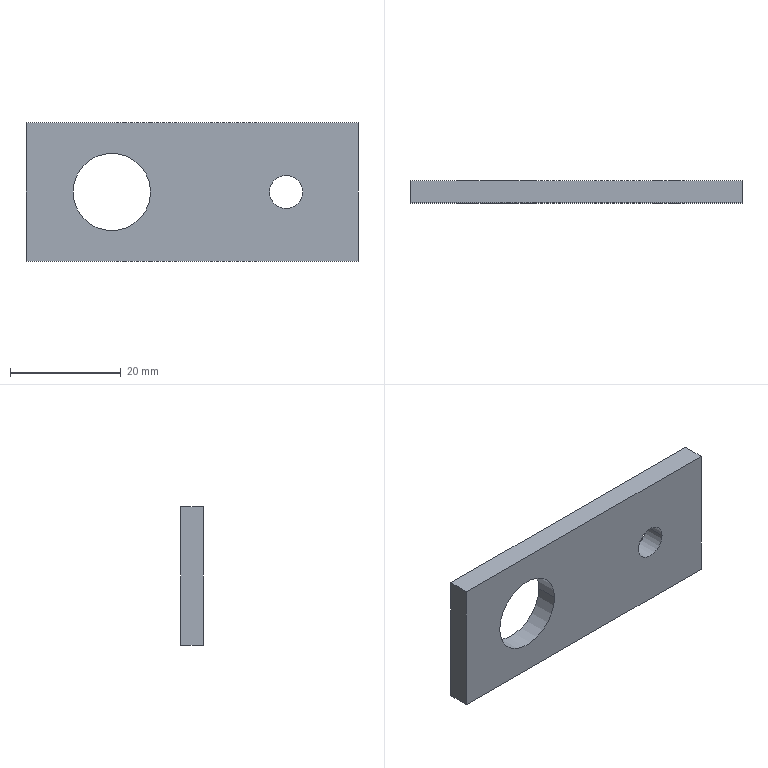Part | STEP file | Connecting plate | 1 solid | 10 faces | box 60 x 4 x 25 mm | volume 5271 mm3 | plane 6 | cylinder 4 | commonest cylinder face diameters 6 x2 14 x2
STEP:
#1=CARTESIAN_POINT('',(-37.49,0.,12.5));
#2=VERTEX_POINT('',#1);
#3=CARTESIAN_POINT('',(-51.49,0.,12.5));
#4=VERTEX_POINT('',#3);
#5=CARTESIAN_POINT('',(-44.49,0.,12.5));
#6=DIRECTION('',(0.,1.,0.));
#7=DIRECTION('',(1.,0.,0.));
#8=AXIS2_PLACEMENT_3D('',#5,#6,#7);
#9=CIRCLE('',#8,7.);
#10=EDGE_CURVE('',#2,#4,#9,.T.);
#11=ORIENTED_EDGE('',*,*,#10,.F.);
#12=CARTESIAN_POINT('',(-37.49,4.,12.5));
#13=VERTEX_POINT('',#12);
#14=CARTESIAN_POINT('',(-37.49,-0.001,12.5));
#15=DIRECTION('',(0.,1.,0.));
#16=VECTOR('',#15,1000.);
#17=LINE('',#14,#16);
#18=EDGE_CURVE('',#2,#13,#17,.T.);
#19=ORIENTED_EDGE('',*,*,#18,.T.);
#20=CARTESIAN_POINT('',(-51.49,4.,12.5));
#21=VERTEX_POINT('',#20);
#22=CARTESIAN_POINT('',(-44.49,4.,12.5));
#23=DIRECTION('',(0.,1.,0.));
#24=DIRECTION('',(-1.,0.,0.));
#25=AXIS2_PLACEMENT_3D('',#22,#23,#24);
#26=CIRCLE('',#25,7.);
#27=EDGE_CURVE('',#13,#21,#26,.T.);
#28=ORIENTED_EDGE('',*,*,#27,.T.);
#29=CARTESIAN_POINT('',(-51.49,-0.001,12.5));
#30=DIRECTION('',(0.,1.,0.));
#31=VECTOR('',#30,1000.);
#32=LINE('',#29,#31);
#33=EDGE_CURVE('',#4,#21,#32,.T.);
#34=ORIENTED_EDGE('',*,*,#33,.F.);
#35=EDGE_LOOP('',(#11,#19,#28,#34));
#36=FACE_OUTER_BOUND('',#35,.T.);
#37=CARTESIAN_POINT('',(-44.49,-0.001,12.5));
#38=DIRECTION('',(0.,1.,0.));
#39=DIRECTION('',(-1.,0.,0.));
#40=AXIS2_PLACEMENT_3D('',#37,#38,#39);
#41=CYLINDRICAL_SURFACE('',#40,7.);
#42=ADVANCED_FACE('',(#36),#41,.F.);
#43=CARTESIAN_POINT('',(-10.,0.,12.5));
#44=VERTEX_POINT('',#43);
#45=CARTESIAN_POINT('',(-16.,0.,12.5));
#46=VERTEX_POINT('',#45);
#47=CARTESIAN_POINT('',(-13.,0.,12.5));
#48=DIRECTION('',(0.,1.,0.));
#49=DIRECTION('',(1.,0.,0.));
#50=AXIS2_PLACEMENT_3D('',#47,#48,#49);
#51=CIRCLE('',#50,3.);
#52=EDGE_CURVE('',#44,#46,#51,.T.);
#53=ORIENTED_EDGE('',*,*,#52,.F.);
#54=CARTESIAN_POINT('',(-10.,4.,12.5));
#55=VERTEX_POINT('',#54);
#56=CARTESIAN_POINT('',(-10.,-0.001,12.5));
#57=DIRECTION('',(0.,1.,0.));
#58=VECTOR('',#57,1000.);
#59=LINE('',#56,#58);
#60=EDGE_CURVE('',#44,#55,#59,.T.);
#61=ORIENTED_EDGE('',*,*,#60,.T.);
#62=CARTESIAN_POINT('',(-16.,4.,12.5));
#63=VERTEX_POINT('',#62);
#64=CARTESIAN_POINT('',(-13.,4.,12.5));
#65=DIRECTION('',(0.,1.,0.));
#66=DIRECTION('',(-1.,0.,0.));
#67=AXIS2_PLACEMENT_3D('',#64,#65,#66);
#68=CIRCLE('',#67,3.);
#69=EDGE_CURVE('',#55,#63,#68,.T.);
#70=ORIENTED_EDGE('',*,*,#69,.T.);
#71=CARTESIAN_POINT('',(-16.,-0.001,12.5));
#72=DIRECTION('',(0.,1.,0.));
#73=VECTOR('',#72,1000.);
#74=LINE('',#71,#73);
#75=EDGE_CURVE('',#46,#63,#74,.T.);
#76=ORIENTED_EDGE('',*,*,#75,.F.);
#77=EDGE_LOOP('',(#53,#61,#70,#76));
#78=FACE_OUTER_BOUND('',#77,.T.);
#79=CARTESIAN_POINT('',(-13.,-0.001,12.5));
#80=DIRECTION('',(0.,1.,0.));
#81=DIRECTION('',(-1.,0.,0.));
#82=AXIS2_PLACEMENT_3D('',#79,#80,#81);
#83=CYLINDRICAL_SURFACE('',#82,3.);
#84=ADVANCED_FACE('',(#78),#83,.F.);
#85=CARTESIAN_POINT('',(-44.49,4.,12.5));
#86=DIRECTION('',(0.,1.,0.));
#87=DIRECTION('',(-1.,0.,0.));
#88=AXIS2_PLACEMENT_3D('',#85,#86,#87);
#89=CIRCLE('',#88,7.);
#90=EDGE_CURVE('',#21,#13,#89,.T.);
#91=ORIENTED_EDGE('',*,*,#90,.F.);
#92=ORIENTED_EDGE('',*,*,#27,.F.);
#93=EDGE_LOOP('',(#91,#92));
#94=FACE_BOUND('',#93,.T.);
#95=CARTESIAN_POINT('',(-13.,4.,12.5));
#96=DIRECTION('',(0.,1.,0.));
#97=DIRECTION('',(-1.,0.,0.));
#98=AXIS2_PLACEMENT_3D('',#95,#96,#97);
#99=CIRCLE('',#98,3.);
#100=EDGE_CURVE('',#63,#55,#99,.T.);
#101=ORIENTED_EDGE('',*,*,#100,.F.);
#102=ORIENTED_EDGE('',*,*,#69,.F.);
#103=EDGE_LOOP('',(#101,#102));
#104=FACE_BOUND('',#103,.T.);
#105=CARTESIAN_POINT('',(0.,4.,0.));
#106=VERTEX_POINT('',#105);
#107=CARTESIAN_POINT('',(-60.,4.,0.));
#108=VERTEX_POINT('',#107);
#109=CARTESIAN_POINT('',(0.,4.,0.));
#110=DIRECTION('',(-1.,0.,0.));
#111=VECTOR('',#110,1000.);
#112=LINE('',#109,#111);
#113=EDGE_CURVE('',#106,#108,#112,.T.);
#114=ORIENTED_EDGE('',*,*,#113,.T.);
#115=CARTESIAN_POINT('',(-60.,4.,25.));
#116=VERTEX_POINT('',#115);
#117=CARTESIAN_POINT('',(-60.,4.,25.));
#118=DIRECTION('',(0.,0.,-1.));
#119=VECTOR('',#118,1000.);
#120=LINE('',#117,#119);
#121=EDGE_CURVE('',#116,#108,#120,.T.);
#122=ORIENTED_EDGE('',*,*,#121,.F.);
#123=CARTESIAN_POINT('',(0.,4.,25.));
#124=VERTEX_POINT('',#123);
#125=CARTESIAN_POINT('',(0.,4.,25.));
#126=DIRECTION('',(-1.,0.,0.));
#127=VECTOR('',#126,1000.);
#128=LINE('',#125,#127);
#129=EDGE_CURVE('',#124,#116,#128,.T.);
#130=ORIENTED_EDGE('',*,*,#129,.F.);
#131=CARTESIAN_POINT('',(0.,4.,25.));
#132=DIRECTION('',(0.,0.,-1.));
#133=VECTOR('',#132,1000.);
#134=LINE('',#131,#133);
#135=EDGE_CURVE('',#124,#106,#134,.T.);
#136=ORIENTED_EDGE('',*,*,#135,.T.);
#137=EDGE_LOOP('',(#114,#122,#130,#136));
#138=FACE_OUTER_BOUND('',#137,.T.);
#139=CARTESIAN_POINT('',(0.,4.,25.));
#140=DIRECTION('',(0.,-1.,0.));
#141=DIRECTION('',(1.,0.,0.));
#142=AXIS2_PLACEMENT_3D('',#139,#140,#141);
#143=PLANE('',#142);
#144=ADVANCED_FACE('',(#94,#104,#138),#143,.F.);
#145=CARTESIAN_POINT('',(-60.,0.,0.));
#146=VERTEX_POINT('',#145);
#147=CARTESIAN_POINT('',(-60.,0.,0.));
#148=DIRECTION('',(0.,1.,0.));
#149=VECTOR('',#148,1000.);
#150=LINE('',#147,#149);
#151=EDGE_CURVE('',#146,#108,#150,.T.);
#152=ORIENTED_EDGE('',*,*,#151,.F.);
#153=CARTESIAN_POINT('',(-60.,0.,25.));
#154=VERTEX_POINT('',#153);
#155=CARTESIAN_POINT('',(-60.,0.,25.));
#156=DIRECTION('',(0.,0.,-1.));
#157=VECTOR('',#156,1000.);
#158=LINE('',#155,#157);
#159=EDGE_CURVE('',#154,#146,#158,.T.);
#160=ORIENTED_EDGE('',*,*,#159,.F.);
#161=CARTESIAN_POINT('',(-60.,0.,25.));
#162=DIRECTION('',(0.,1.,0.));
#163=VECTOR('',#162,1000.);
#164=LINE('',#161,#163);
#165=EDGE_CURVE('',#154,#116,#164,.T.);
#166=ORIENTED_EDGE('',*,*,#165,.T.);
#167=ORIENTED_EDGE('',*,*,#121,.T.);
#168=EDGE_LOOP('',(#152,#160,#166,#167));
#169=FACE_OUTER_BOUND('',#168,.T.);
#170=CARTESIAN_POINT('',(-60.,0.,25.));
#171=DIRECTION('',(-1.,0.,0.));
#172=DIRECTION('',(0.,0.,1.));
#173=AXIS2_PLACEMENT_3D('',#170,#171,#172);
#174=PLANE('',#173);
#175=ADVANCED_FACE('',(#169),#174,.T.);
#176=CARTESIAN_POINT('',(-44.49,0.,12.5));
#177=DIRECTION('',(0.,1.,0.));
#178=DIRECTION('',(1.,0.,0.));
#179=AXIS2_PLACEMENT_3D('',#176,#177,#178);
#180=CIRCLE('',#179,7.);
#181=EDGE_CURVE('',#4,#2,#180,.T.);
#182=ORIENTED_EDGE('',*,*,#181,.T.);
#183=ORIENTED_EDGE('',*,*,#10,.T.);
#184=EDGE_LOOP('',(#182,#183));
#185=FACE_BOUND('',#184,.T.);
#186=CARTESIAN_POINT('',(-13.,0.,12.5));
#187=DIRECTION('',(0.,1.,0.));
#188=DIRECTION('',(1.,0.,0.));
#189=AXIS2_PLACEMENT_3D('',#186,#187,#188);
#190=CIRCLE('',#189,3.);
#191=EDGE_CURVE('',#46,#44,#190,.T.);
#192=ORIENTED_EDGE('',*,*,#191,.T.);
#193=ORIENTED_EDGE('',*,*,#52,.T.);
#194=EDGE_LOOP('',(#192,#193));
#195=FACE_BOUND('',#194,.T.);
#196=CARTESIAN_POINT('',(0.,0.,0.));
#197=VERTEX_POINT('',#196);
#198=CARTESIAN_POINT('',(0.,0.,0.));
#199=DIRECTION('',(-1.,0.,0.));
#200=VECTOR('',#199,1000.);
#201=LINE('',#198,#200);
#202=EDGE_CURVE('',#197,#146,#201,.T.);
#203=ORIENTED_EDGE('',*,*,#202,.F.);
#204=CARTESIAN_POINT('',(0.,0.,25.));
#205=VERTEX_POINT('',#204);
#206=CARTESIAN_POINT('',(0.,0.,25.));
#207=DIRECTION('',(0.,0.,-1.));
#208=VECTOR('',#207,1000.);
#209=LINE('',#206,#208);
#210=EDGE_CURVE('',#205,#197,#209,.T.);
#211=ORIENTED_EDGE('',*,*,#210,.F.);
#212=CARTESIAN_POINT('',(0.,0.,25.));
#213=DIRECTION('',(-1.,0.,0.));
#214=VECTOR('',#213,1000.);
#215=LINE('',#212,#214);
#216=EDGE_CURVE('',#205,#154,#215,.T.);
#217=ORIENTED_EDGE('',*,*,#216,.T.);
#218=ORIENTED_EDGE('',*,*,#159,.T.);
#219=EDGE_LOOP('',(#203,#211,#217,#218));
#220=FACE_OUTER_BOUND('',#219,.T.);
#221=CARTESIAN_POINT('',(0.,0.,25.));
#222=DIRECTION('',(0.,-1.,0.));
#223=DIRECTION('',(1.,0.,0.));
#224=AXIS2_PLACEMENT_3D('',#221,#222,#223);
#225=PLANE('',#224);
#226=ADVANCED_FACE('',(#185,#195,#220),#225,.T.);
#227=CARTESIAN_POINT('',(0.,4.,0.));
#228=DIRECTION('',(0.,-1.,0.));
#229=VECTOR('',#228,1000.);
#230=LINE('',#227,#229);
#231=EDGE_CURVE('',#106,#197,#230,.T.);
#232=ORIENTED_EDGE('',*,*,#231,.F.);
#233=ORIENTED_EDGE('',*,*,#135,.F.);
#234=CARTESIAN_POINT('',(0.,4.,25.));
#235=DIRECTION('',(0.,-1.,0.));
#236=VECTOR('',#235,1000.);
#237=LINE('',#234,#236);
#238=EDGE_CURVE('',#124,#205,#237,.T.);
#239=ORIENTED_EDGE('',*,*,#238,.T.);
#240=ORIENTED_EDGE('',*,*,#210,.T.);
#241=EDGE_LOOP('',(#232,#233,#239,#240));
#242=FACE_OUTER_BOUND('',#241,.T.);
#243=CARTESIAN_POINT('',(0.,4.,25.));
#244=DIRECTION('',(1.,0.,0.));
#245=DIRECTION('',(0.,1.,0.));
#246=AXIS2_PLACEMENT_3D('',#243,#244,#245);
#247=PLANE('',#246);
#248=ADVANCED_FACE('',(#242),#247,.T.);
#249=ORIENTED_EDGE('',*,*,#129,.T.);
#250=ORIENTED_EDGE('',*,*,#165,.F.);
#251=ORIENTED_EDGE('',*,*,#216,.F.);
#252=ORIENTED_EDGE('',*,*,#238,.F.);
#253=EDGE_LOOP('',(#249,#250,#251,#252));
#254=FACE_OUTER_BOUND('',#253,.T.);
#255=CARTESIAN_POINT('',(0.,0.,25.));
#256=DIRECTION('',(0.,0.,-1.));
#257=DIRECTION('',(-1.,0.,0.));
#258=AXIS2_PLACEMENT_3D('',#255,#256,#257);
#259=PLANE('',#258);
#260=ADVANCED_FACE('',(#254),#259,.F.);
#261=ORIENTED_EDGE('',*,*,#113,.F.);
#262=ORIENTED_EDGE('',*,*,#231,.T.);
#263=ORIENTED_EDGE('',*,*,#202,.T.);
#264=ORIENTED_EDGE('',*,*,#151,.T.);
#265=EDGE_LOOP('',(#261,#262,#263,#264));
#266=FACE_OUTER_BOUND('',#265,.T.);
#267=CARTESIAN_POINT('',(0.,0.,0.));
#268=DIRECTION('',(0.,0.,-1.));
#269=DIRECTION('',(-1.,0.,0.));
#270=AXIS2_PLACEMENT_3D('',#267,#268,#269);
#271=PLANE('',#270);
#272=ADVANCED_FACE('',(#266),#271,.T.);
#273=ORIENTED_EDGE('',*,*,#60,.F.);
#274=ORIENTED_EDGE('',*,*,#191,.F.);
#275=ORIENTED_EDGE('',*,*,#75,.T.);
#276=ORIENTED_EDGE('',*,*,#100,.T.);
#277=EDGE_LOOP('',(#273,#274,#275,#276));
#278=FACE_OUTER_BOUND('',#277,.T.);
#279=CARTESIAN_POINT('',(-13.,-0.001,12.5));
#280=DIRECTION('',(0.,1.,0.));
#281=DIRECTION('',(-1.,0.,0.));
#282=AXIS2_PLACEMENT_3D('',#279,#280,#281);
#283=CYLINDRICAL_SURFACE('',#282,3.);
#284=ADVANCED_FACE('',(#278),#283,.F.);
#285=ORIENTED_EDGE('',*,*,#18,.F.);
#286=ORIENTED_EDGE('',*,*,#181,.F.);
#287=ORIENTED_EDGE('',*,*,#33,.T.);
#288=ORIENTED_EDGE('',*,*,#90,.T.);
#289=EDGE_LOOP('',(#285,#286,#287,#288));
#290=FACE_OUTER_BOUND('',#289,.T.);
#291=CARTESIAN_POINT('',(-44.49,-0.001,12.5));
#292=DIRECTION('',(0.,1.,0.));
#293=DIRECTION('',(-1.,0.,0.));
#294=AXIS2_PLACEMENT_3D('',#291,#292,#293);
#295=CYLINDRICAL_SURFACE('',#294,7.);
#296=ADVANCED_FACE('',(#290),#295,.F.);
#297=CLOSED_SHELL('',(#42,#84,#144,#175,#226,#248,#260,#272,#284,#296));
#298=MANIFOLD_SOLID_BREP('',#297);
#299=CARTESIAN_POINT('',(0.,0.,0.));
#300=DIRECTION('',(0.,0.,1.));
#301=DIRECTION('',(1.,0.,0.));
#302=AXIS2_PLACEMENT_3D('',#299,#300,#301);
#303=(LENGTH_UNIT()NAMED_UNIT(*)SI_UNIT(.MILLI.,.METRE.));
#304=UNCERTAINTY_MEASURE_WITH_UNIT(LENGTH_MEASURE(0.00001),#303,'','');
#305=(NAMED_UNIT(*)PLANE_ANGLE_UNIT()SI_UNIT($,.RADIAN.));
#306=(NAMED_UNIT(*)SI_UNIT($,.STERADIAN.)SOLID_ANGLE_UNIT());
#307=(GEOMETRIC_REPRESENTATION_CONTEXT(3)GLOBAL_UNCERTAINTY_ASSIGNED_CONTEXT((#304))GLOBAL_UNIT_ASSIGNED_CONTEXT((#303,#305,#306))REPRESENTATION_CONTEXT('',''));
#308=ADVANCED_BREP_SHAPE_REPRESENTATION('',(#298,#302),#307);